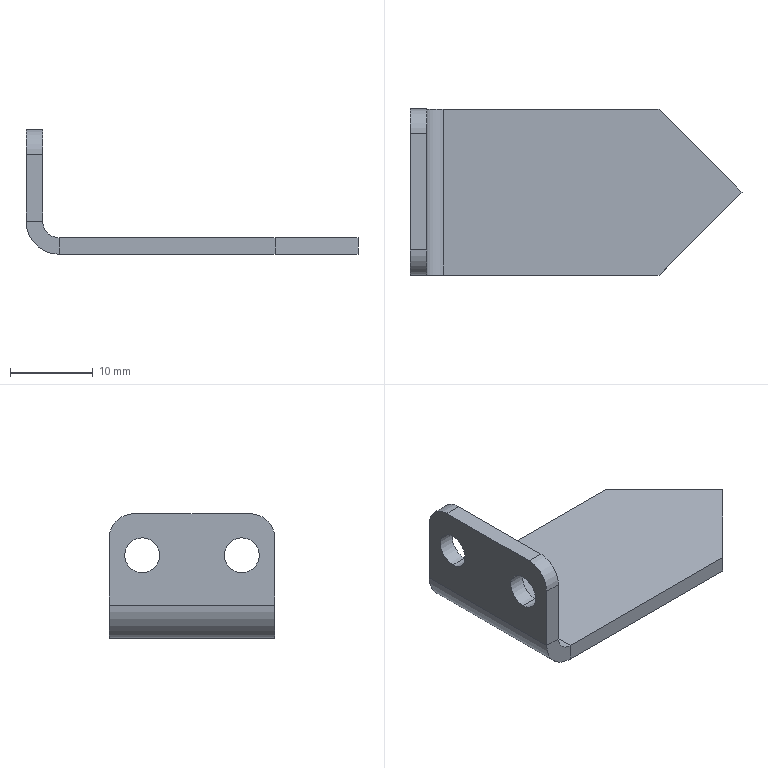Part | SolidWorks | features EdgeFlange 1, Fillet 1, FlatPattern 1, HoleWzd 1, ICE 1, SMBaseFlange 1, SheetMetal 1 | 1 solid | 21 faces | box 40 x 20 x 15 mm | volume 1805 mm3 | plane 13 | cylinder 8 | commonest cylinder face diameters 4.2 x4 6 x2 4 x1 8 x1
STEP:
#1=CARTESIAN_POINT('',(2.,4.,10.1));
#2=VERTEX_POINT('',#1);
#3=CARTESIAN_POINT('',(2.,4.,5.9));
#4=VERTEX_POINT('',#3);
#5=CARTESIAN_POINT('',(2.,4.,8.));
#6=DIRECTION('',(1.,0.,0.));
#7=DIRECTION('',(0.,0.,-1.));
#8=AXIS2_PLACEMENT_3D('',#5,#6,#7);
#9=CIRCLE('',#8,2.1);
#10=EDGE_CURVE('',#2,#4,#9,.T.);
#11=ORIENTED_EDGE('',*,*,#10,.T.);
#12=CARTESIAN_POINT('',(0.,4.,5.9));
#13=VERTEX_POINT('',#12);
#14=CARTESIAN_POINT('',(0.,4.,5.9));
#15=DIRECTION('',(-1.,0.,0.));
#16=VECTOR('',#15,1000.);
#17=LINE('',#14,#16);
#18=EDGE_CURVE('',#4,#13,#17,.T.);
#19=ORIENTED_EDGE('',*,*,#18,.T.);
#20=CARTESIAN_POINT('',(0.,4.,10.1));
#21=VERTEX_POINT('',#20);
#22=CARTESIAN_POINT('',(0.,4.,8.));
#23=DIRECTION('',(-1.,0.,0.));
#24=DIRECTION('',(0.,0.,1.));
#25=AXIS2_PLACEMENT_3D('',#22,#23,#24);
#26=CIRCLE('',#25,2.1);
#27=EDGE_CURVE('',#13,#21,#26,.T.);
#28=ORIENTED_EDGE('',*,*,#27,.T.);
#29=CARTESIAN_POINT('',(0.,4.,10.1));
#30=DIRECTION('',(-1.,0.,0.));
#31=VECTOR('',#30,1000.);
#32=LINE('',#29,#31);
#33=EDGE_CURVE('',#2,#21,#32,.T.);
#34=ORIENTED_EDGE('',*,*,#33,.F.);
#35=EDGE_LOOP('',(#11,#19,#28,#34));
#36=FACE_OUTER_BOUND('',#35,.T.);
#37=CARTESIAN_POINT('',(0.,4.,8.));
#38=DIRECTION('',(-1.,0.,0.));
#39=DIRECTION('',(0.,0.,1.));
#40=AXIS2_PLACEMENT_3D('',#37,#38,#39);
#41=CYLINDRICAL_SURFACE('',#40,2.1);
#42=ADVANCED_FACE('',(#36),#41,.F.);
#43=CARTESIAN_POINT('',(2.,16.,10.1));
#44=VERTEX_POINT('',#43);
#45=CARTESIAN_POINT('',(2.,16.,5.9));
#46=VERTEX_POINT('',#45);
#47=CARTESIAN_POINT('',(2.,16.,8.));
#48=DIRECTION('',(1.,0.,0.));
#49=DIRECTION('',(0.,0.,-1.));
#50=AXIS2_PLACEMENT_3D('',#47,#48,#49);
#51=CIRCLE('',#50,2.1);
#52=EDGE_CURVE('',#44,#46,#51,.T.);
#53=ORIENTED_EDGE('',*,*,#52,.T.);
#54=CARTESIAN_POINT('',(0.,16.,5.9));
#55=VERTEX_POINT('',#54);
#56=CARTESIAN_POINT('',(0.,16.,5.9));
#57=DIRECTION('',(-1.,0.,0.));
#58=VECTOR('',#57,1000.);
#59=LINE('',#56,#58);
#60=EDGE_CURVE('',#46,#55,#59,.T.);
#61=ORIENTED_EDGE('',*,*,#60,.T.);
#62=CARTESIAN_POINT('',(0.,16.,10.1));
#63=VERTEX_POINT('',#62);
#64=CARTESIAN_POINT('',(0.,16.,8.));
#65=DIRECTION('',(-1.,0.,0.));
#66=DIRECTION('',(0.,0.,1.));
#67=AXIS2_PLACEMENT_3D('',#64,#65,#66);
#68=CIRCLE('',#67,2.1);
#69=EDGE_CURVE('',#55,#63,#68,.T.);
#70=ORIENTED_EDGE('',*,*,#69,.T.);
#71=CARTESIAN_POINT('',(0.,16.,10.1));
#72=DIRECTION('',(-1.,0.,0.));
#73=VECTOR('',#72,1000.);
#74=LINE('',#71,#73);
#75=EDGE_CURVE('',#44,#63,#74,.T.);
#76=ORIENTED_EDGE('',*,*,#75,.F.);
#77=EDGE_LOOP('',(#53,#61,#70,#76));
#78=FACE_OUTER_BOUND('',#77,.T.);
#79=CARTESIAN_POINT('',(0.,16.,8.));
#80=DIRECTION('',(-1.,0.,0.));
#81=DIRECTION('',(0.,0.,1.));
#82=AXIS2_PLACEMENT_3D('',#79,#80,#81);
#83=CYLINDRICAL_SURFACE('',#82,2.1);
#84=ADVANCED_FACE('',(#78),#83,.F.);
#85=CARTESIAN_POINT('',(40.,10.,-2.));
#86=VERTEX_POINT('',#85);
#87=CARTESIAN_POINT('',(30.,20.,-2.));
#88=VERTEX_POINT('',#87);
#89=CARTESIAN_POINT('',(25.,25.,-2.));
#90=DIRECTION('',(-0.7071,0.7071,0.));
#91=VECTOR('',#90,1000.);
#92=LINE('',#89,#91);
#93=EDGE_CURVE('',#86,#88,#92,.T.);
#94=ORIENTED_EDGE('',*,*,#93,.F.);
#95=CARTESIAN_POINT('',(30.,0.,-2.));
#96=VERTEX_POINT('',#95);
#97=CARTESIAN_POINT('',(40.,10.,-2.));
#98=DIRECTION('',(-0.7071,-0.7071,0.));
#99=VECTOR('',#98,1000.);
#100=LINE('',#97,#99);
#101=EDGE_CURVE('',#86,#96,#100,.T.);
#102=ORIENTED_EDGE('',*,*,#101,.T.);
#103=CARTESIAN_POINT('',(4.,0.,-2.));
#104=VERTEX_POINT('',#103);
#105=CARTESIAN_POINT('',(0.,0.,-2.));
#106=DIRECTION('',(1.,0.,0.));
#107=VECTOR('',#106,1000.);
#108=LINE('',#105,#107);
#109=EDGE_CURVE('',#104,#96,#108,.T.);
#110=ORIENTED_EDGE('',*,*,#109,.F.);
#111=CARTESIAN_POINT('',(4.,20.,-2.));
#112=VERTEX_POINT('',#111);
#113=CARTESIAN_POINT('',(4.,0.,-2.));
#114=DIRECTION('',(0.,1.,0.));
#115=VECTOR('',#114,1000.);
#116=LINE('',#113,#115);
#117=EDGE_CURVE('',#104,#112,#116,.T.);
#118=ORIENTED_EDGE('',*,*,#117,.T.);
#119=CARTESIAN_POINT('',(0.,20.,-2.));
#120=DIRECTION('',(-1.,0.,0.));
#121=VECTOR('',#120,1000.);
#122=LINE('',#119,#121);
#123=EDGE_CURVE('',#88,#112,#122,.T.);
#124=ORIENTED_EDGE('',*,*,#123,.F.);
#125=EDGE_LOOP('',(#94,#102,#110,#118,#124));
#126=FACE_OUTER_BOUND('',#125,.T.);
#127=CARTESIAN_POINT('',(0.,0.,-2.));
#128=DIRECTION('',(0.,0.,-1.));
#129=DIRECTION('',(-1.,0.,0.));
#130=AXIS2_PLACEMENT_3D('',#127,#128,#129);
#131=PLANE('',#130);
#132=ADVANCED_FACE('',(#126),#131,.T.);
#133=CARTESIAN_POINT('',(40.,10.,0.));
#134=VERTEX_POINT('',#133);
#135=CARTESIAN_POINT('',(30.,0.,0.));
#136=VERTEX_POINT('',#135);
#137=CARTESIAN_POINT('',(40.,10.,0.));
#138=DIRECTION('',(-0.7071,-0.7071,0.));
#139=VECTOR('',#138,1000.);
#140=LINE('',#137,#139);
#141=EDGE_CURVE('',#134,#136,#140,.T.);
#142=ORIENTED_EDGE('',*,*,#141,.F.);
#143=CARTESIAN_POINT('',(30.,20.,0.));
#144=VERTEX_POINT('',#143);
#145=CARTESIAN_POINT('',(25.,25.,0.));
#146=DIRECTION('',(-0.7071,0.7071,0.));
#147=VECTOR('',#146,1000.);
#148=LINE('',#145,#147);
#149=EDGE_CURVE('',#134,#144,#148,.T.);
#150=ORIENTED_EDGE('',*,*,#149,.T.);
#151=CARTESIAN_POINT('',(4.,20.,0.));
#152=VERTEX_POINT('',#151);
#153=CARTESIAN_POINT('',(0.,20.,0.));
#154=DIRECTION('',(-1.,0.,0.));
#155=VECTOR('',#154,1000.);
#156=LINE('',#153,#155);
#157=EDGE_CURVE('',#144,#152,#156,.T.);
#158=ORIENTED_EDGE('',*,*,#157,.T.);
#159=CARTESIAN_POINT('',(4.,0.,0.));
#160=VERTEX_POINT('',#159);
#161=CARTESIAN_POINT('',(4.,0.,0.));
#162=DIRECTION('',(0.,1.,0.));
#163=VECTOR('',#162,1000.);
#164=LINE('',#161,#163);
#165=EDGE_CURVE('',#160,#152,#164,.T.);
#166=ORIENTED_EDGE('',*,*,#165,.F.);
#167=CARTESIAN_POINT('',(0.,0.,0.));
#168=DIRECTION('',(1.,0.,0.));
#169=VECTOR('',#168,1000.);
#170=LINE('',#167,#169);
#171=EDGE_CURVE('',#160,#136,#170,.T.);
#172=ORIENTED_EDGE('',*,*,#171,.T.);
#173=EDGE_LOOP('',(#142,#150,#158,#166,#172));
#174=FACE_OUTER_BOUND('',#173,.T.);
#175=CARTESIAN_POINT('',(0.,0.,0.));
#176=DIRECTION('',(0.,0.,-1.));
#177=DIRECTION('',(-1.,0.,0.));
#178=AXIS2_PLACEMENT_3D('',#175,#176,#177);
#179=PLANE('',#178);
#180=ADVANCED_FACE('',(#174),#179,.F.);
#181=ORIENTED_EDGE('',*,*,#109,.T.);
#182=CARTESIAN_POINT('',(30.,0.,0.));
#183=DIRECTION('',(0.,0.,-1.));
#184=VECTOR('',#183,1000.);
#185=LINE('',#182,#184);
#186=EDGE_CURVE('',#136,#96,#185,.T.);
#187=ORIENTED_EDGE('',*,*,#186,.F.);
#188=ORIENTED_EDGE('',*,*,#171,.F.);
#189=CARTESIAN_POINT('',(4.,0.,0.));
#190=DIRECTION('',(0.,0.,-1.));
#191=VECTOR('',#190,1000.);
#192=LINE('',#189,#191);
#193=EDGE_CURVE('',#160,#104,#192,.T.);
#194=ORIENTED_EDGE('',*,*,#193,.T.);
#195=EDGE_LOOP('',(#181,#187,#188,#194));
#196=FACE_OUTER_BOUND('',#195,.T.);
#197=CARTESIAN_POINT('',(0.,0.,-2.));
#198=DIRECTION('',(0.,-1.,0.));
#199=DIRECTION('',(0.,0.,-1.));
#200=AXIS2_PLACEMENT_3D('',#197,#198,#199);
#201=PLANE('',#200);
#202=ADVANCED_FACE('',(#196),#201,.T.);
#203=ORIENTED_EDGE('',*,*,#157,.F.);
#204=CARTESIAN_POINT('',(30.,20.,-2.));
#205=DIRECTION('',(0.,0.,1.));
#206=VECTOR('',#205,1000.);
#207=LINE('',#204,#206);
#208=EDGE_CURVE('',#88,#144,#207,.T.);
#209=ORIENTED_EDGE('',*,*,#208,.F.);
#210=ORIENTED_EDGE('',*,*,#123,.T.);
#211=CARTESIAN_POINT('',(4.,20.,0.));
#212=DIRECTION('',(0.,0.,-1.));
#213=VECTOR('',#212,1000.);
#214=LINE('',#211,#213);
#215=EDGE_CURVE('',#152,#112,#214,.T.);
#216=ORIENTED_EDGE('',*,*,#215,.F.);
#217=EDGE_LOOP('',(#203,#209,#210,#216));
#218=FACE_OUTER_BOUND('',#217,.T.);
#219=CARTESIAN_POINT('',(0.,20.,-2.));
#220=DIRECTION('',(0.,1.,0.));
#221=DIRECTION('',(0.,0.,1.));
#222=AXIS2_PLACEMENT_3D('',#219,#220,#221);
#223=PLANE('',#222);
#224=ADVANCED_FACE('',(#218),#223,.T.);
#225=CARTESIAN_POINT('',(2.,20.,2.));
#226=VERTEX_POINT('',#225);
#227=CARTESIAN_POINT('',(0.,20.,2.));
#228=VERTEX_POINT('',#227);
#229=CARTESIAN_POINT('',(0.,20.,2.));
#230=DIRECTION('',(-1.,0.,0.));
#231=VECTOR('',#230,1000.);
#232=LINE('',#229,#231);
#233=EDGE_CURVE('',#226,#228,#232,.T.);
#234=ORIENTED_EDGE('',*,*,#233,.F.);
#235=CARTESIAN_POINT('',(4.,20.,2.));
#236=DIRECTION('',(0.,1.,0.));
#237=DIRECTION('',(0.,0.,-1.));
#238=AXIS2_PLACEMENT_3D('',#235,#236,#237);
#239=CIRCLE('',#238,2.);
#240=EDGE_CURVE('',#152,#226,#239,.T.);
#241=ORIENTED_EDGE('',*,*,#240,.F.);
#242=ORIENTED_EDGE('',*,*,#215,.T.);
#243=CARTESIAN_POINT('',(4.,20.,2.));
#244=DIRECTION('',(0.,1.,0.));
#245=DIRECTION('',(0.,0.,-1.));
#246=AXIS2_PLACEMENT_3D('',#243,#244,#245);
#247=CIRCLE('',#246,4.);
#248=EDGE_CURVE('',#112,#228,#247,.T.);
#249=ORIENTED_EDGE('',*,*,#248,.T.);
#250=EDGE_LOOP('',(#234,#241,#242,#249));
#251=FACE_OUTER_BOUND('',#250,.T.);
#252=CARTESIAN_POINT('',(4.,20.,2.));
#253=DIRECTION('',(0.,1.,0.));
#254=DIRECTION('',(0.,0.,1.));
#255=AXIS2_PLACEMENT_3D('',#252,#253,#254);
#256=PLANE('',#255);
#257=ADVANCED_FACE('',(#251),#256,.T.);
#258=CARTESIAN_POINT('',(2.,0.,2.));
#259=VERTEX_POINT('',#258);
#260=CARTESIAN_POINT('',(4.,0.,2.));
#261=DIRECTION('',(0.,-1.,0.));
#262=DIRECTION('',(0.,0.,-1.));
#263=AXIS2_PLACEMENT_3D('',#260,#261,#262);
#264=CIRCLE('',#263,2.);
#265=EDGE_CURVE('',#259,#160,#264,.T.);
#266=ORIENTED_EDGE('',*,*,#265,.F.);
#267=CARTESIAN_POINT('',(0.,0.,2.));
#268=VERTEX_POINT('',#267);
#269=CARTESIAN_POINT('',(2.,0.,2.));
#270=DIRECTION('',(-1.,0.,0.));
#271=VECTOR('',#270,1000.);
#272=LINE('',#269,#271);
#273=EDGE_CURVE('',#259,#268,#272,.T.);
#274=ORIENTED_EDGE('',*,*,#273,.T.);
#275=CARTESIAN_POINT('',(4.,0.,2.));
#276=DIRECTION('',(0.,-1.,0.));
#277=DIRECTION('',(0.,0.,-1.));
#278=AXIS2_PLACEMENT_3D('',#275,#276,#277);
#279=CIRCLE('',#278,4.);
#280=EDGE_CURVE('',#268,#104,#279,.T.);
#281=ORIENTED_EDGE('',*,*,#280,.T.);
#282=ORIENTED_EDGE('',*,*,#193,.F.);
#283=EDGE_LOOP('',(#266,#274,#281,#282));
#284=FACE_OUTER_BOUND('',#283,.T.);
#285=CARTESIAN_POINT('',(4.,0.,2.));
#286=DIRECTION('',(0.,1.,0.));
#287=DIRECTION('',(0.,0.,1.));
#288=AXIS2_PLACEMENT_3D('',#285,#286,#287);
#289=PLANE('',#288);
#290=ADVANCED_FACE('',(#284),#289,.F.);
#291=ORIENTED_EDGE('',*,*,#117,.F.);
#292=ORIENTED_EDGE('',*,*,#280,.F.);
#293=CARTESIAN_POINT('',(0.,20.,2.));
#294=DIRECTION('',(0.,1.,0.));
#295=VECTOR('',#294,1000.);
#296=LINE('',#293,#295);
#297=EDGE_CURVE('',#268,#228,#296,.T.);
#298=ORIENTED_EDGE('',*,*,#297,.T.);
#299=ORIENTED_EDGE('',*,*,#248,.F.);
#300=EDGE_LOOP('',(#291,#292,#298,#299));
#301=FACE_OUTER_BOUND('',#300,.T.);
#302=CARTESIAN_POINT('',(4.,0.,2.));
#303=DIRECTION('',(0.,-1.,0.));
#304=DIRECTION('',(-1.,0.,0.));
#305=AXIS2_PLACEMENT_3D('',#302,#303,#304);
#306=CYLINDRICAL_SURFACE('',#305,4.);
#307=ADVANCED_FACE('',(#301),#306,.T.);
#308=ORIENTED_EDGE('',*,*,#165,.T.);
#309=ORIENTED_EDGE('',*,*,#240,.T.);
#310=CARTESIAN_POINT('',(2.,20.,2.));
#311=DIRECTION('',(0.,-1.,0.));
#312=VECTOR('',#311,1000.);
#313=LINE('',#310,#312);
#314=EDGE_CURVE('',#226,#259,#313,.T.);
#315=ORIENTED_EDGE('',*,*,#314,.T.);
#316=ORIENTED_EDGE('',*,*,#265,.T.);
#317=EDGE_LOOP('',(#308,#309,#315,#316));
#318=FACE_OUTER_BOUND('',#317,.T.);
#319=CARTESIAN_POINT('',(4.,0.,2.));
#320=DIRECTION('',(0.,-1.,0.));
#321=DIRECTION('',(-1.,0.,0.));
#322=AXIS2_PLACEMENT_3D('',#319,#320,#321);
#323=CYLINDRICAL_SURFACE('',#322,2.);
#324=ADVANCED_FACE('',(#318),#323,.F.);
#325=CARTESIAN_POINT('',(0.,20.,10.));
#326=VERTEX_POINT('',#325);
#327=CARTESIAN_POINT('',(0.,20.,0.));
#328=DIRECTION('',(0.,0.,-1.));
#329=VECTOR('',#328,1000.);
#330=LINE('',#327,#329);
#331=EDGE_CURVE('',#326,#228,#330,.T.);
#332=ORIENTED_EDGE('',*,*,#331,.F.);
#333=CARTESIAN_POINT('',(2.,20.,10.));
#334=VERTEX_POINT('',#333);
#335=CARTESIAN_POINT('',(0.,20.,10.));
#336=DIRECTION('',(1.,0.,0.));
#337=VECTOR('',#336,1000.);
#338=LINE('',#335,#337);
#339=EDGE_CURVE('',#326,#334,#338,.T.);
#340=ORIENTED_EDGE('',*,*,#339,.T.);
#341=CARTESIAN_POINT('',(2.,20.,0.));
#342=DIRECTION('',(0.,0.,-1.));
#343=VECTOR('',#342,1000.);
#344=LINE('',#341,#343);
#345=EDGE_CURVE('',#334,#226,#344,.T.);
#346=ORIENTED_EDGE('',*,*,#345,.T.);
#347=ORIENTED_EDGE('',*,*,#233,.T.);
#348=EDGE_LOOP('',(#332,#340,#346,#347));
#349=FACE_OUTER_BOUND('',#348,.T.);
#350=CARTESIAN_POINT('',(0.,20.,0.));
#351=DIRECTION('',(0.,-1.,0.));
#352=DIRECTION('',(0.,0.,-1.));
#353=AXIS2_PLACEMENT_3D('',#350,#351,#352);
#354=PLANE('',#353);
#355=ADVANCED_FACE('',(#349),#354,.F.);
#356=CARTESIAN_POINT('',(2.,0.,10.));
#357=VERTEX_POINT('',#356);
#358=CARTESIAN_POINT('',(2.,0.,13.));
#359=DIRECTION('',(0.,0.,1.));
#360=VECTOR('',#359,1000.);
#361=LINE('',#358,#360);
#362=EDGE_CURVE('',#259,#357,#361,.T.);
#363=ORIENTED_EDGE('',*,*,#362,.T.);
#364=CARTESIAN_POINT('',(0.,0.,10.));
#365=VERTEX_POINT('',#364);
#366=CARTESIAN_POINT('',(0.,0.,10.));
#367=DIRECTION('',(-1.,0.,0.));
#368=VECTOR('',#367,1000.);
#369=LINE('',#366,#368);
#370=EDGE_CURVE('',#357,#365,#369,.T.);
#371=ORIENTED_EDGE('',*,*,#370,.T.);
#372=CARTESIAN_POINT('',(0.,0.,0.));
#373=DIRECTION('',(0.,0.,1.));
#374=VECTOR('',#373,1000.);
#375=LINE('',#372,#374);
#376=EDGE_CURVE('',#268,#365,#375,.T.);
#377=ORIENTED_EDGE('',*,*,#376,.F.);
#378=ORIENTED_EDGE('',*,*,#273,.F.);
#379=EDGE_LOOP('',(#363,#371,#377,#378));
#380=FACE_OUTER_BOUND('',#379,.T.);
#381=CARTESIAN_POINT('',(0.,0.,13.));
#382=DIRECTION('',(0.,1.,0.));
#383=DIRECTION('',(0.,0.,1.));
#384=AXIS2_PLACEMENT_3D('',#381,#382,#383);
#385=PLANE('',#384);
#386=ADVANCED_FACE('',(#380),#385,.F.);
#387=CARTESIAN_POINT('',(0.,4.,8.));
#388=DIRECTION('',(-1.,0.,0.));
#389=DIRECTION('',(0.,0.,1.));
#390=AXIS2_PLACEMENT_3D('',#387,#388,#389);
#391=CIRCLE('',#390,2.1);
#392=EDGE_CURVE('',#21,#13,#391,.T.);
#393=ORIENTED_EDGE('',*,*,#392,.F.);
#394=ORIENTED_EDGE('',*,*,#27,.F.);
#395=EDGE_LOOP('',(#393,#394));
#396=FACE_BOUND('',#395,.T.);
#397=CARTESIAN_POINT('',(0.,16.,8.));
#398=DIRECTION('',(-1.,0.,0.));
#399=DIRECTION('',(0.,0.,1.));
#400=AXIS2_PLACEMENT_3D('',#397,#398,#399);
#401=CIRCLE('',#400,2.1);
#402=EDGE_CURVE('',#63,#55,#401,.T.);
#403=ORIENTED_EDGE('',*,*,#402,.F.);
#404=ORIENTED_EDGE('',*,*,#69,.F.);
#405=EDGE_LOOP('',(#403,#404));
#406=FACE_BOUND('',#405,.T.);
#407=CARTESIAN_POINT('',(0.,3.,13.));
#408=VERTEX_POINT('',#407);
#409=CARTESIAN_POINT('',(0.,17.,13.));
#410=VERTEX_POINT('',#409);
#411=CARTESIAN_POINT('',(0.,0.,13.));
#412=DIRECTION('',(0.,1.,0.));
#413=VECTOR('',#412,1000.);
#414=LINE('',#411,#413);
#415=EDGE_CURVE('',#408,#410,#414,.T.);
#416=ORIENTED_EDGE('',*,*,#415,.T.);
#417=CARTESIAN_POINT('',(0.,17.,10.));
#418=DIRECTION('',(-1.,0.,0.));
#419=DIRECTION('',(0.,0.,-1.));
#420=AXIS2_PLACEMENT_3D('',#417,#418,#419);
#421=CIRCLE('',#420,3.);
#422=EDGE_CURVE('',#410,#326,#421,.T.);
#423=ORIENTED_EDGE('',*,*,#422,.T.);
#424=ORIENTED_EDGE('',*,*,#331,.T.);
#425=ORIENTED_EDGE('',*,*,#297,.F.);
#426=ORIENTED_EDGE('',*,*,#376,.T.);
#427=CARTESIAN_POINT('',(0.,3.,10.));
#428=DIRECTION('',(-1.,0.,0.));
#429=DIRECTION('',(0.,0.,-1.));
#430=AXIS2_PLACEMENT_3D('',#427,#428,#429);
#431=CIRCLE('',#430,3.);
#432=EDGE_CURVE('',#365,#408,#431,.T.);
#433=ORIENTED_EDGE('',*,*,#432,.T.);
#434=EDGE_LOOP('',(#416,#423,#424,#425,#426,#433));
#435=FACE_OUTER_BOUND('',#434,.T.);
#436=CARTESIAN_POINT('',(0.,0.,0.));
#437=DIRECTION('',(1.,0.,0.));
#438=DIRECTION('',(0.,0.,-1.));
#439=AXIS2_PLACEMENT_3D('',#436,#437,#438);
#440=PLANE('',#439);
#441=ADVANCED_FACE('',(#396,#406,#435),#440,.F.);
#442=ORIENTED_EDGE('',*,*,#10,.F.);
#443=CARTESIAN_POINT('',(2.,4.,8.));
#444=DIRECTION('',(1.,0.,0.));
#445=DIRECTION('',(0.,0.,-1.));
#446=AXIS2_PLACEMENT_3D('',#443,#444,#445);
#447=CIRCLE('',#446,2.1);
#448=EDGE_CURVE('',#4,#2,#447,.T.);
#449=ORIENTED_EDGE('',*,*,#448,.F.);
#450=EDGE_LOOP('',(#442,#449));
#451=FACE_BOUND('',#450,.T.);
#452=ORIENTED_EDGE('',*,*,#52,.F.);
#453=CARTESIAN_POINT('',(2.,16.,8.));
#454=DIRECTION('',(1.,0.,0.));
#455=DIRECTION('',(0.,0.,-1.));
#456=AXIS2_PLACEMENT_3D('',#453,#454,#455);
#457=CIRCLE('',#456,2.1);
#458=EDGE_CURVE('',#46,#44,#457,.T.);
#459=ORIENTED_EDGE('',*,*,#458,.F.);
#460=EDGE_LOOP('',(#452,#459));
#461=FACE_BOUND('',#460,.T.);
#462=ORIENTED_EDGE('',*,*,#345,.F.);
#463=CARTESIAN_POINT('',(2.,17.,13.));
#464=VERTEX_POINT('',#463);
#465=CARTESIAN_POINT('',(2.,17.,10.));
#466=DIRECTION('',(1.,0.,0.));
#467=DIRECTION('',(0.,0.,-1.));
#468=AXIS2_PLACEMENT_3D('',#465,#466,#467);
#469=CIRCLE('',#468,3.);
#470=EDGE_CURVE('',#334,#464,#469,.T.);
#471=ORIENTED_EDGE('',*,*,#470,.T.);
#472=CARTESIAN_POINT('',(2.,3.,13.));
#473=VERTEX_POINT('',#472);
#474=CARTESIAN_POINT('',(2.,20.,13.));
#475=DIRECTION('',(0.,1.,0.));
#476=VECTOR('',#475,1000.);
#477=LINE('',#474,#476);
#478=EDGE_CURVE('',#473,#464,#477,.T.);
#479=ORIENTED_EDGE('',*,*,#478,.F.);
#480=CARTESIAN_POINT('',(2.,3.,10.));
#481=DIRECTION('',(1.,0.,0.));
#482=DIRECTION('',(0.,0.,-1.));
#483=AXIS2_PLACEMENT_3D('',#480,#481,#482);
#484=CIRCLE('',#483,3.);
#485=EDGE_CURVE('',#473,#357,#484,.T.);
#486=ORIENTED_EDGE('',*,*,#485,.T.);
#487=ORIENTED_EDGE('',*,*,#362,.F.);
#488=ORIENTED_EDGE('',*,*,#314,.F.);
#489=EDGE_LOOP('',(#462,#471,#479,#486,#487,#488));
#490=FACE_OUTER_BOUND('',#489,.T.);
#491=CARTESIAN_POINT('',(2.,0.,0.));
#492=DIRECTION('',(1.,0.,0.));
#493=DIRECTION('',(0.,0.,-1.));
#494=AXIS2_PLACEMENT_3D('',#491,#492,#493);
#495=PLANE('',#494);
#496=ADVANCED_FACE('',(#451,#461,#490),#495,.T.);
#497=ORIENTED_EDGE('',*,*,#478,.T.);
#498=CARTESIAN_POINT('',(0.,17.,13.));
#499=DIRECTION('',(-1.,0.,0.));
#500=VECTOR('',#499,1000.);
#501=LINE('',#498,#500);
#502=EDGE_CURVE('',#464,#410,#501,.T.);
#503=ORIENTED_EDGE('',*,*,#502,.T.);
#504=ORIENTED_EDGE('',*,*,#415,.F.);
#505=CARTESIAN_POINT('',(0.,3.,13.));
#506=DIRECTION('',(1.,0.,0.));
#507=VECTOR('',#506,1000.);
#508=LINE('',#505,#507);
#509=EDGE_CURVE('',#408,#473,#508,.T.);
#510=ORIENTED_EDGE('',*,*,#509,.T.);
#511=EDGE_LOOP('',(#497,#503,#504,#510));
#512=FACE_OUTER_BOUND('',#511,.T.);
#513=CARTESIAN_POINT('',(0.,20.,13.));
#514=DIRECTION('',(0.,0.,-1.));
#515=DIRECTION('',(-1.,0.,0.));
#516=AXIS2_PLACEMENT_3D('',#513,#514,#515);
#517=PLANE('',#516);
#518=ADVANCED_FACE('',(#512),#517,.F.);
#519=ORIENTED_EDGE('',*,*,#60,.F.);
#520=ORIENTED_EDGE('',*,*,#458,.T.);
#521=ORIENTED_EDGE('',*,*,#75,.T.);
#522=ORIENTED_EDGE('',*,*,#402,.T.);
#523=EDGE_LOOP('',(#519,#520,#521,#522));
#524=FACE_OUTER_BOUND('',#523,.T.);
#525=CARTESIAN_POINT('',(0.,16.,8.));
#526=DIRECTION('',(-1.,0.,0.));
#527=DIRECTION('',(0.,0.,1.));
#528=AXIS2_PLACEMENT_3D('',#525,#526,#527);
#529=CYLINDRICAL_SURFACE('',#528,2.1);
#530=ADVANCED_FACE('',(#524),#529,.F.);
#531=ORIENTED_EDGE('',*,*,#18,.F.);
#532=ORIENTED_EDGE('',*,*,#448,.T.);
#533=ORIENTED_EDGE('',*,*,#33,.T.);
#534=ORIENTED_EDGE('',*,*,#392,.T.);
#535=EDGE_LOOP('',(#531,#532,#533,#534));
#536=FACE_OUTER_BOUND('',#535,.T.);
#537=CARTESIAN_POINT('',(0.,4.,8.));
#538=DIRECTION('',(-1.,0.,0.));
#539=DIRECTION('',(0.,0.,1.));
#540=AXIS2_PLACEMENT_3D('',#537,#538,#539);
#541=CYLINDRICAL_SURFACE('',#540,2.1);
#542=ADVANCED_FACE('',(#536),#541,.F.);
#543=ORIENTED_EDGE('',*,*,#422,.F.);
#544=ORIENTED_EDGE('',*,*,#502,.F.);
#545=ORIENTED_EDGE('',*,*,#470,.F.);
#546=ORIENTED_EDGE('',*,*,#339,.F.);
#547=EDGE_LOOP('',(#543,#544,#545,#546));
#548=FACE_OUTER_BOUND('',#547,.T.);
#549=CARTESIAN_POINT('',(0.,17.,10.));
#550=DIRECTION('',(1.,0.,0.));
#551=DIRECTION('',(0.,0.,-1.));
#552=AXIS2_PLACEMENT_3D('',#549,#550,#551);
#553=CYLINDRICAL_SURFACE('',#552,3.);
#554=ADVANCED_FACE('',(#548),#553,.T.);
#555=ORIENTED_EDGE('',*,*,#432,.F.);
#556=ORIENTED_EDGE('',*,*,#370,.F.);
#557=ORIENTED_EDGE('',*,*,#485,.F.);
#558=ORIENTED_EDGE('',*,*,#509,.F.);
#559=EDGE_LOOP('',(#555,#556,#557,#558));
#560=FACE_OUTER_BOUND('',#559,.T.);
#561=CARTESIAN_POINT('',(0.,3.,10.));
#562=DIRECTION('',(1.,0.,0.));
#563=DIRECTION('',(0.,0.,-1.));
#564=AXIS2_PLACEMENT_3D('',#561,#562,#563);
#565=CYLINDRICAL_SURFACE('',#564,3.);
#566=ADVANCED_FACE('',(#560),#565,.T.);
#567=ORIENTED_EDGE('',*,*,#93,.T.);
#568=ORIENTED_EDGE('',*,*,#208,.T.);
#569=ORIENTED_EDGE('',*,*,#149,.F.);
#570=CARTESIAN_POINT('',(40.,10.,-2.));
#571=DIRECTION('',(0.,0.,1.));
#572=VECTOR('',#571,1000.);
#573=LINE('',#570,#572);
#574=EDGE_CURVE('',#86,#134,#573,.T.);
#575=ORIENTED_EDGE('',*,*,#574,.F.);
#576=EDGE_LOOP('',(#567,#568,#569,#575));
#577=FACE_OUTER_BOUND('',#576,.T.);
#578=CARTESIAN_POINT('',(25.,25.,-2.));
#579=DIRECTION('',(-0.7071,-0.7071,0.));
#580=DIRECTION('',(-0.7071,0.7071,0.));
#581=AXIS2_PLACEMENT_3D('',#578,#579,#580);
#582=PLANE('',#581);
#583=ADVANCED_FACE('',(#577),#582,.F.);
#584=ORIENTED_EDGE('',*,*,#574,.T.);
#585=ORIENTED_EDGE('',*,*,#141,.T.);
#586=ORIENTED_EDGE('',*,*,#186,.T.);
#587=ORIENTED_EDGE('',*,*,#101,.F.);
#588=EDGE_LOOP('',(#584,#585,#586,#587));
#589=FACE_OUTER_BOUND('',#588,.T.);
#590=CARTESIAN_POINT('',(40.,10.,0.));
#591=DIRECTION('',(0.7071,-0.7071,0.));
#592=DIRECTION('',(-0.7071,-0.7071,0.));
#593=AXIS2_PLACEMENT_3D('',#590,#591,#592);
#594=PLANE('',#593);
#595=ADVANCED_FACE('',(#589),#594,.T.);
#596=CLOSED_SHELL('',(#42,#84,#132,#180,#202,#224,#257,#290,#307,#324,#355,#386,#441,#496,#518,#530,#542,#554,#566,#583,#595));
#597=MANIFOLD_SOLID_BREP('',#596);
#598=CARTESIAN_POINT('',(0.,0.,0.));
#599=DIRECTION('',(0.,0.,1.));
#600=DIRECTION('',(1.,0.,0.));
#601=AXIS2_PLACEMENT_3D('',#598,#599,#600);
#602=(LENGTH_UNIT()NAMED_UNIT(*)SI_UNIT(.MILLI.,.METRE.));
#603=UNCERTAINTY_MEASURE_WITH_UNIT(LENGTH_MEASURE(0.00001),#602,'','');
#604=(NAMED_UNIT(*)PLANE_ANGLE_UNIT()SI_UNIT($,.RADIAN.));
#605=(NAMED_UNIT(*)SI_UNIT($,.STERADIAN.)SOLID_ANGLE_UNIT());
#606=(GEOMETRIC_REPRESENTATION_CONTEXT(3)GLOBAL_UNCERTAINTY_ASSIGNED_CONTEXT((#603))GLOBAL_UNIT_ASSIGNED_CONTEXT((#602,#604,#605))REPRESENTATION_CONTEXT('',''));
#607=ADVANCED_BREP_SHAPE_REPRESENTATION('',(#597,#601),#606);